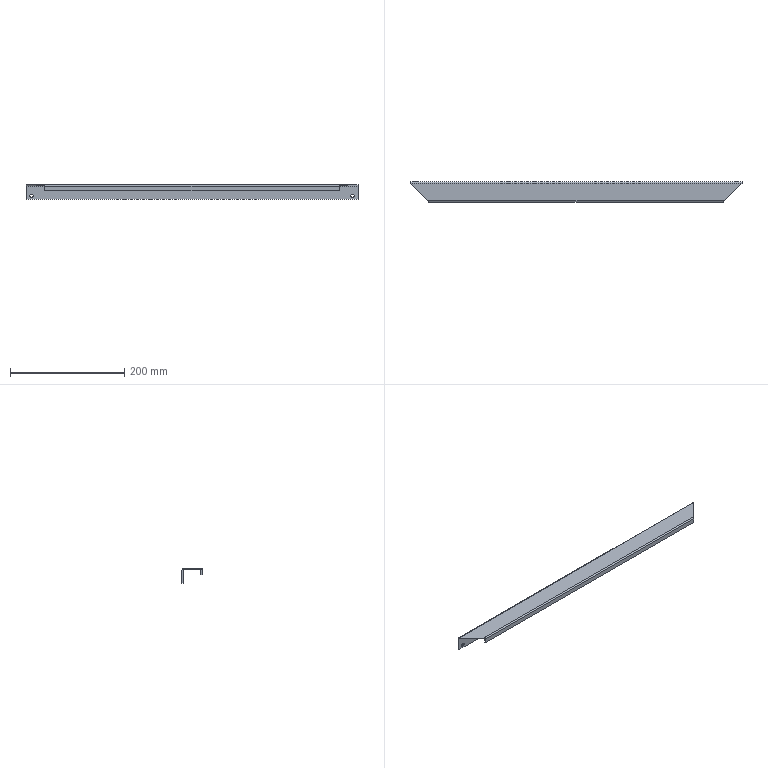Part | STEP file | Right Door Frame 3 | 1 solid | 24 faces | box 580 x 35 x 25 mm | volume 72212 mm3 | plane 16 | cylinder 8 | commonest cylinder face diameters 6 x4 0.2 x2 4.2 x2
STEP:
#1=CARTESIAN_POINT('',(-44.225,-2.,-11.695));
#2=VERTEX_POINT('',#1);
#3=CARTESIAN_POINT('',(-44.225,-2.,-5.695));
#4=VERTEX_POINT('',#3);
#5=CARTESIAN_POINT('',(-44.225,-2.,-8.695));
#6=DIRECTION('',(0.,1.,0.));
#7=DIRECTION('',(0.,0.,1.));
#8=AXIS2_PLACEMENT_3D('',#5,#6,#7);
#9=CIRCLE('',#8,3.);
#10=EDGE_CURVE('',#2,#4,#9,.T.);
#11=ORIENTED_EDGE('',*,*,#10,.F.);
#12=CARTESIAN_POINT('',(-44.225,0.,-11.695));
#13=VERTEX_POINT('',#12);
#14=CARTESIAN_POINT('',(-44.225,-10.,-11.695));
#15=DIRECTION('',(0.,1.,0.));
#16=VECTOR('',#15,1000.);
#17=LINE('',#14,#16);
#18=EDGE_CURVE('',#2,#13,#17,.T.);
#19=ORIENTED_EDGE('',*,*,#18,.T.);
#20=CARTESIAN_POINT('',(-44.225,0.,-5.695));
#21=VERTEX_POINT('',#20);
#22=CARTESIAN_POINT('',(-44.225,0.,-8.695));
#23=DIRECTION('',(0.,-1.,0.));
#24=DIRECTION('',(0.,0.,1.));
#25=AXIS2_PLACEMENT_3D('',#22,#23,#24);
#26=CIRCLE('',#25,3.);
#27=EDGE_CURVE('',#21,#13,#26,.T.);
#28=ORIENTED_EDGE('',*,*,#27,.F.);
#29=CARTESIAN_POINT('',(-44.225,-10.,-5.695));
#30=DIRECTION('',(0.,1.,0.));
#31=VECTOR('',#30,1000.);
#32=LINE('',#29,#31);
#33=EDGE_CURVE('',#4,#21,#32,.T.);
#34=ORIENTED_EDGE('',*,*,#33,.F.);
#35=EDGE_LOOP('',(#11,#19,#28,#34));
#36=FACE_OUTER_BOUND('',#35,.T.);
#37=CARTESIAN_POINT('',(-44.225,-10.,-8.695));
#38=DIRECTION('',(0.,1.,0.));
#39=DIRECTION('',(0.,0.,1.));
#40=AXIS2_PLACEMENT_3D('',#37,#38,#39);
#41=CYLINDRICAL_SURFACE('',#40,3.);
#42=ADVANCED_FACE('',(#36),#41,.F.);
#43=CARTESIAN_POINT('',(516.775,-2.,-11.695));
#44=VERTEX_POINT('',#43);
#45=CARTESIAN_POINT('',(516.775,-2.,-5.695));
#46=VERTEX_POINT('',#45);
#47=CARTESIAN_POINT('',(516.775,-2.,-8.695));
#48=DIRECTION('',(0.,1.,0.));
#49=DIRECTION('',(0.,0.,1.));
#50=AXIS2_PLACEMENT_3D('',#47,#48,#49);
#51=CIRCLE('',#50,3.);
#52=EDGE_CURVE('',#44,#46,#51,.T.);
#53=ORIENTED_EDGE('',*,*,#52,.F.);
#54=CARTESIAN_POINT('',(516.775,0.,-11.695));
#55=VERTEX_POINT('',#54);
#56=CARTESIAN_POINT('',(516.775,-10.,-11.695));
#57=DIRECTION('',(0.,1.,0.));
#58=VECTOR('',#57,1000.);
#59=LINE('',#56,#58);
#60=EDGE_CURVE('',#44,#55,#59,.T.);
#61=ORIENTED_EDGE('',*,*,#60,.T.);
#62=CARTESIAN_POINT('',(516.775,0.,-5.695));
#63=VERTEX_POINT('',#62);
#64=CARTESIAN_POINT('',(516.775,0.,-8.695));
#65=DIRECTION('',(0.,-1.,0.));
#66=DIRECTION('',(0.,0.,1.));
#67=AXIS2_PLACEMENT_3D('',#64,#65,#66);
#68=CIRCLE('',#67,3.);
#69=EDGE_CURVE('',#63,#55,#68,.T.);
#70=ORIENTED_EDGE('',*,*,#69,.F.);
#71=CARTESIAN_POINT('',(516.775,-10.,-5.695));
#72=DIRECTION('',(0.,1.,0.));
#73=VECTOR('',#72,1000.);
#74=LINE('',#71,#73);
#75=EDGE_CURVE('',#46,#63,#74,.T.);
#76=ORIENTED_EDGE('',*,*,#75,.F.);
#77=EDGE_LOOP('',(#53,#61,#70,#76));
#78=FACE_OUTER_BOUND('',#77,.T.);
#79=CARTESIAN_POINT('',(516.775,-10.,-8.695));
#80=DIRECTION('',(0.,1.,0.));
#81=DIRECTION('',(0.,0.,1.));
#82=AXIS2_PLACEMENT_3D('',#79,#80,#81);
#83=CYLINDRICAL_SURFACE('',#82,3.);
#84=ADVANCED_FACE('',(#78),#83,.F.);
#85=CARTESIAN_POINT('',(526.275,-2.1,10.305));
#86=VERTEX_POINT('',#85);
#87=CARTESIAN_POINT('',(-53.725,-2.1,10.305));
#88=VERTEX_POINT('',#87);
#89=CARTESIAN_POINT('',(0.,-2.1,10.305));
#90=DIRECTION('',(-1.,0.,0.));
#91=VECTOR('',#90,1000.);
#92=LINE('',#89,#91);
#93=EDGE_CURVE('',#86,#88,#92,.T.);
#94=ORIENTED_EDGE('',*,*,#93,.T.);
#95=CARTESIAN_POINT('',(-53.725,-2.2,10.305));
#96=VERTEX_POINT('',#95);
#97=CARTESIAN_POINT('',(-53.725,-2.,10.305));
#98=DIRECTION('',(0.,1.,0.));
#99=VECTOR('',#98,1000.);
#100=LINE('',#97,#99);
#101=EDGE_CURVE('',#96,#88,#100,.T.);
#102=ORIENTED_EDGE('',*,*,#101,.F.);
#103=CARTESIAN_POINT('',(-20.925,-35.,10.305));
#104=VERTEX_POINT('',#103);
#105=CARTESIAN_POINT('',(-53.725,-2.2,10.305));
#106=DIRECTION('',(0.7071,-0.7071,0.));
#107=VECTOR('',#106,1000.);
#108=LINE('',#105,#107);
#109=EDGE_CURVE('',#96,#104,#108,.T.);
#110=ORIENTED_EDGE('',*,*,#109,.T.);
#111=CARTESIAN_POINT('',(-20.925,-32.9,10.305));
#112=VERTEX_POINT('',#111);
#113=CARTESIAN_POINT('',(-20.925,0.,10.305));
#114=DIRECTION('',(0.,1.,0.));
#115=VECTOR('',#114,1000.);
#116=LINE('',#113,#115);
#117=EDGE_CURVE('',#104,#112,#116,.T.);
#118=ORIENTED_EDGE('',*,*,#117,.T.);
#119=CARTESIAN_POINT('',(493.475,-32.9,10.305));
#120=VERTEX_POINT('',#119);
#121=CARTESIAN_POINT('',(0.,-32.9,10.305));
#122=DIRECTION('',(1.,0.,0.));
#123=VECTOR('',#122,1000.);
#124=LINE('',#121,#123);
#125=EDGE_CURVE('',#112,#120,#124,.T.);
#126=ORIENTED_EDGE('',*,*,#125,.T.);
#127=CARTESIAN_POINT('',(493.475,-35.,10.305));
#128=VERTEX_POINT('',#127);
#129=CARTESIAN_POINT('',(493.475,0.,10.305));
#130=DIRECTION('',(0.,-1.,0.));
#131=VECTOR('',#130,1000.);
#132=LINE('',#129,#131);
#133=EDGE_CURVE('',#120,#128,#132,.T.);
#134=ORIENTED_EDGE('',*,*,#133,.T.);
#135=CARTESIAN_POINT('',(526.275,-2.2,10.305));
#136=VERTEX_POINT('',#135);
#137=CARTESIAN_POINT('',(493.475,-35.,10.305));
#138=DIRECTION('',(0.7071,0.7071,0.));
#139=VECTOR('',#138,1000.);
#140=LINE('',#137,#139);
#141=EDGE_CURVE('',#128,#136,#140,.T.);
#142=ORIENTED_EDGE('',*,*,#141,.T.);
#143=CARTESIAN_POINT('',(526.275,-35.,10.305));
#144=DIRECTION('',(0.,-1.,0.));
#145=VECTOR('',#144,1000.);
#146=LINE('',#143,#145);
#147=EDGE_CURVE('',#86,#136,#146,.T.);
#148=ORIENTED_EDGE('',*,*,#147,.F.);
#149=EDGE_LOOP('',(#94,#102,#110,#118,#126,#134,#142,#148));
#150=FACE_OUTER_BOUND('',#149,.T.);
#151=CARTESIAN_POINT('',(0.,0.,10.305));
#152=DIRECTION('',(0.,0.,1.));
#153=DIRECTION('',(0.,-1.,0.));
#154=AXIS2_PLACEMENT_3D('',#151,#152,#153);
#155=PLANE('',#154);
#156=ADVANCED_FACE('',(#150),#155,.T.);
#157=ORIENTED_EDGE('',*,*,#93,.F.);
#158=CARTESIAN_POINT('',(526.275,0.,8.205));
#159=VERTEX_POINT('',#158);
#160=CARTESIAN_POINT('',(526.275,-2.1,8.205));
#161=DIRECTION('',(-1.,0.,0.));
#162=DIRECTION('',(0.,0.,1.));
#163=AXIS2_PLACEMENT_3D('',#160,#161,#162);
#164=CIRCLE('',#163,2.1);
#165=EDGE_CURVE('',#86,#159,#164,.T.);
#166=ORIENTED_EDGE('',*,*,#165,.T.);
#167=CARTESIAN_POINT('',(-53.725,0.,8.205));
#168=VERTEX_POINT('',#167);
#169=CARTESIAN_POINT('',(-53.725,0.,8.205));
#170=DIRECTION('',(-1.,0.,0.));
#171=VECTOR('',#170,1000.);
#172=LINE('',#169,#171);
#173=EDGE_CURVE('',#159,#168,#172,.T.);
#174=ORIENTED_EDGE('',*,*,#173,.T.);
#175=CARTESIAN_POINT('',(-53.725,-2.1,8.205));
#176=DIRECTION('',(1.,0.,0.));
#177=DIRECTION('',(0.,0.,1.));
#178=AXIS2_PLACEMENT_3D('',#175,#176,#177);
#179=CIRCLE('',#178,2.1);
#180=EDGE_CURVE('',#168,#88,#179,.T.);
#181=ORIENTED_EDGE('',*,*,#180,.T.);
#182=EDGE_LOOP('',(#157,#166,#174,#181));
#183=FACE_OUTER_BOUND('',#182,.T.);
#184=CARTESIAN_POINT('',(-53.725,-2.1,8.205));
#185=DIRECTION('',(-1.,0.,0.));
#186=DIRECTION('',(0.,0.,1.));
#187=AXIS2_PLACEMENT_3D('',#184,#185,#186);
#188=CYLINDRICAL_SURFACE('',#187,2.1);
#189=ADVANCED_FACE('',(#183),#188,.T.);
#190=CARTESIAN_POINT('',(493.475,-35.,8.305));
#191=VERTEX_POINT('',#190);
#192=CARTESIAN_POINT('',(493.475,-35.,10.305));
#193=DIRECTION('',(0.,0.,1.));
#194=VECTOR('',#193,1000.);
#195=LINE('',#192,#194);
#196=EDGE_CURVE('',#191,#128,#195,.T.);
#197=ORIENTED_EDGE('',*,*,#196,.F.);
#198=CARTESIAN_POINT('',(526.275,-2.2,8.305));
#199=VERTEX_POINT('',#198);
#200=CARTESIAN_POINT('',(526.275,-2.2,8.305));
#201=DIRECTION('',(-0.7071,-0.7071,0.));
#202=VECTOR('',#201,1000.);
#203=LINE('',#200,#202);
#204=EDGE_CURVE('',#199,#191,#203,.T.);
#205=ORIENTED_EDGE('',*,*,#204,.F.);
#206=CARTESIAN_POINT('',(526.275,-2.2,10.305));
#207=DIRECTION('',(0.,0.,-1.));
#208=VECTOR('',#207,1000.);
#209=LINE('',#206,#208);
#210=EDGE_CURVE('',#136,#199,#209,.T.);
#211=ORIENTED_EDGE('',*,*,#210,.F.);
#212=ORIENTED_EDGE('',*,*,#141,.F.);
#213=EDGE_LOOP('',(#197,#205,#211,#212));
#214=FACE_OUTER_BOUND('',#213,.T.);
#215=CARTESIAN_POINT('',(526.275,-2.2,10.305));
#216=DIRECTION('',(-0.7071,0.7071,0.));
#217=DIRECTION('',(-0.7071,-0.7071,0.));
#218=AXIS2_PLACEMENT_3D('',#215,#216,#217);
#219=PLANE('',#218);
#220=ADVANCED_FACE('',(#214),#219,.F.);
#221=CARTESIAN_POINT('',(493.475,-34.998,8.305));
#222=VERTEX_POINT('',#221);
#223=CARTESIAN_POINT('',(493.475,-32.9,8.305));
#224=DIRECTION('',(0.,-1.,0.));
#225=VECTOR('',#224,1000.);
#226=LINE('',#223,#225);
#227=EDGE_CURVE('',#222,#191,#226,.T.);
#228=ORIENTED_EDGE('',*,*,#227,.T.);
#229=ORIENTED_EDGE('',*,*,#196,.T.);
#230=ORIENTED_EDGE('',*,*,#133,.F.);
#231=CARTESIAN_POINT('',(493.475,-32.9,8.205));
#232=DIRECTION('',(1.,0.,0.));
#233=DIRECTION('',(0.,0.,1.));
#234=AXIS2_PLACEMENT_3D('',#231,#232,#233);
#235=CIRCLE('',#234,2.1);
#236=EDGE_CURVE('',#120,#222,#235,.T.);
#237=ORIENTED_EDGE('',*,*,#236,.T.);
#238=EDGE_LOOP('',(#228,#229,#230,#237));
#239=FACE_OUTER_BOUND('',#238,.T.);
#240=CARTESIAN_POINT('',(493.475,-32.9,8.305));
#241=DIRECTION('',(-1.,0.,0.));
#242=DIRECTION('',(0.,-1.,0.));
#243=AXIS2_PLACEMENT_3D('',#240,#241,#242);
#244=PLANE('',#243);
#245=ADVANCED_FACE('',(#239),#244,.T.);
#246=CARTESIAN_POINT('',(493.475,-35.,8.205));
#247=VERTEX_POINT('',#246);
#248=CARTESIAN_POINT('',(493.475,-32.9,8.205));
#249=DIRECTION('',(1.,0.,0.));
#250=DIRECTION('',(0.,0.,-1.));
#251=AXIS2_PLACEMENT_3D('',#248,#249,#250);
#252=CIRCLE('',#251,2.1);
#253=EDGE_CURVE('',#222,#247,#252,.T.);
#254=ORIENTED_EDGE('',*,*,#253,.F.);
#255=ORIENTED_EDGE('',*,*,#236,.F.);
#256=ORIENTED_EDGE('',*,*,#125,.F.);
#257=CARTESIAN_POINT('',(-20.925,-34.998,8.305));
#258=VERTEX_POINT('',#257);
#259=CARTESIAN_POINT('',(-20.925,-32.9,8.205));
#260=DIRECTION('',(1.,0.,0.));
#261=DIRECTION('',(0.,0.,1.));
#262=AXIS2_PLACEMENT_3D('',#259,#260,#261);
#263=CIRCLE('',#262,2.1);
#264=EDGE_CURVE('',#112,#258,#263,.T.);
#265=ORIENTED_EDGE('',*,*,#264,.T.);
#266=CARTESIAN_POINT('',(-20.925,-35.,8.205));
#267=VERTEX_POINT('',#266);
#268=CARTESIAN_POINT('',(-20.925,-32.9,8.205));
#269=DIRECTION('',(1.,0.,0.));
#270=DIRECTION('',(0.,0.,1.));
#271=AXIS2_PLACEMENT_3D('',#268,#269,#270);
#272=CIRCLE('',#271,2.1);
#273=EDGE_CURVE('',#258,#267,#272,.T.);
#274=ORIENTED_EDGE('',*,*,#273,.T.);
#275=CARTESIAN_POINT('',(-20.925,-35.,8.205));
#276=DIRECTION('',(1.,0.,0.));
#277=VECTOR('',#276,1000.);
#278=LINE('',#275,#277);
#279=EDGE_CURVE('',#267,#247,#278,.T.);
#280=ORIENTED_EDGE('',*,*,#279,.T.);
#281=EDGE_LOOP('',(#254,#255,#256,#265,#274,#280));
#282=FACE_OUTER_BOUND('',#281,.T.);
#283=CARTESIAN_POINT('',(-20.925,-32.9,8.205));
#284=DIRECTION('',(-1.,0.,0.));
#285=DIRECTION('',(0.,0.,1.));
#286=AXIS2_PLACEMENT_3D('',#283,#284,#285);
#287=CYLINDRICAL_SURFACE('',#286,2.1);
#288=ADVANCED_FACE('',(#282),#287,.T.);
#289=ORIENTED_EDGE('',*,*,#117,.F.);
#290=CARTESIAN_POINT('',(-20.925,-35.,8.305));
#291=VERTEX_POINT('',#290);
#292=CARTESIAN_POINT('',(-20.925,-35.,8.305));
#293=DIRECTION('',(0.,0.,-1.));
#294=VECTOR('',#293,1000.);
#295=LINE('',#292,#294);
#296=EDGE_CURVE('',#104,#291,#295,.T.);
#297=ORIENTED_EDGE('',*,*,#296,.T.);
#298=CARTESIAN_POINT('',(-20.925,-35.,8.305));
#299=DIRECTION('',(0.,1.,0.));
#300=VECTOR('',#299,1000.);
#301=LINE('',#298,#300);
#302=EDGE_CURVE('',#291,#258,#301,.T.);
#303=ORIENTED_EDGE('',*,*,#302,.T.);
#304=ORIENTED_EDGE('',*,*,#264,.F.);
#305=EDGE_LOOP('',(#289,#297,#303,#304));
#306=FACE_OUTER_BOUND('',#305,.T.);
#307=CARTESIAN_POINT('',(-20.925,-35.,8.305));
#308=DIRECTION('',(1.,0.,0.));
#309=DIRECTION('',(0.,1.,0.));
#310=AXIS2_PLACEMENT_3D('',#307,#308,#309);
#311=PLANE('',#310);
#312=ADVANCED_FACE('',(#306),#311,.T.);
#313=CARTESIAN_POINT('',(-53.725,-2.2,8.305));
#314=VERTEX_POINT('',#313);
#315=CARTESIAN_POINT('',(-53.725,-2.2,10.305));
#316=DIRECTION('',(0.,0.,1.));
#317=VECTOR('',#316,1000.);
#318=LINE('',#315,#317);
#319=EDGE_CURVE('',#314,#96,#318,.T.);
#320=ORIENTED_EDGE('',*,*,#319,.F.);
#321=CARTESIAN_POINT('',(-20.925,-35.,8.305));
#322=DIRECTION('',(-0.7071,0.7071,0.));
#323=VECTOR('',#322,1000.);
#324=LINE('',#321,#323);
#325=EDGE_CURVE('',#291,#314,#324,.T.);
#326=ORIENTED_EDGE('',*,*,#325,.F.);
#327=ORIENTED_EDGE('',*,*,#296,.F.);
#328=ORIENTED_EDGE('',*,*,#109,.F.);
#329=EDGE_LOOP('',(#320,#326,#327,#328));
#330=FACE_OUTER_BOUND('',#329,.T.);
#331=CARTESIAN_POINT('',(-20.925,-35.,10.305));
#332=DIRECTION('',(0.7071,0.7071,0.));
#333=DIRECTION('',(-0.7071,0.7071,0.));
#334=AXIS2_PLACEMENT_3D('',#331,#332,#333);
#335=PLANE('',#334);
#336=ADVANCED_FACE('',(#330),#335,.F.);
#337=CARTESIAN_POINT('',(526.275,-2.1,8.305));
#338=VERTEX_POINT('',#337);
#339=CARTESIAN_POINT('',(526.275,-2.,8.205));
#340=VERTEX_POINT('',#339);
#341=CARTESIAN_POINT('',(526.275,-2.1,8.205));
#342=DIRECTION('',(-1.,0.,0.));
#343=DIRECTION('',(0.,0.,1.));
#344=AXIS2_PLACEMENT_3D('',#341,#342,#343);
#345=CIRCLE('',#344,0.1);
#346=EDGE_CURVE('',#338,#340,#345,.T.);
#347=ORIENTED_EDGE('',*,*,#346,.T.);
#348=CARTESIAN_POINT('',(526.275,-2.,-14.695));
#349=VERTEX_POINT('',#348);
#350=CARTESIAN_POINT('',(526.275,-2.,-14.695));
#351=DIRECTION('',(0.,0.,-1.));
#352=VECTOR('',#351,1000.);
#353=LINE('',#350,#352);
#354=EDGE_CURVE('',#340,#349,#353,.T.);
#355=ORIENTED_EDGE('',*,*,#354,.T.);
#356=CARTESIAN_POINT('',(526.275,0.,-14.695));
#357=VERTEX_POINT('',#356);
#358=CARTESIAN_POINT('',(526.275,-2.,-14.695));
#359=DIRECTION('',(0.,1.,0.));
#360=VECTOR('',#359,1000.);
#361=LINE('',#358,#360);
#362=EDGE_CURVE('',#349,#357,#361,.T.);
#363=ORIENTED_EDGE('',*,*,#362,.T.);
#364=CARTESIAN_POINT('',(526.275,0.,0.));
#365=DIRECTION('',(0.,0.,-1.));
#366=VECTOR('',#365,1000.);
#367=LINE('',#364,#366);
#368=EDGE_CURVE('',#159,#357,#367,.T.);
#369=ORIENTED_EDGE('',*,*,#368,.F.);
#370=ORIENTED_EDGE('',*,*,#165,.F.);
#371=ORIENTED_EDGE('',*,*,#147,.T.);
#372=ORIENTED_EDGE('',*,*,#210,.T.);
#373=CARTESIAN_POINT('',(526.275,0.,8.305));
#374=DIRECTION('',(0.,1.,0.));
#375=VECTOR('',#374,1000.);
#376=LINE('',#373,#375);
#377=EDGE_CURVE('',#199,#338,#376,.T.);
#378=ORIENTED_EDGE('',*,*,#377,.T.);
#379=EDGE_LOOP('',(#347,#355,#363,#369,#370,#371,#372,#378));
#380=FACE_OUTER_BOUND('',#379,.T.);
#381=CARTESIAN_POINT('',(526.275,-2.1,8.205));
#382=DIRECTION('',(1.,0.,0.));
#383=DIRECTION('',(0.,0.,-1.));
#384=AXIS2_PLACEMENT_3D('',#381,#382,#383);
#385=PLANE('',#384);
#386=ADVANCED_FACE('',(#380),#385,.T.);
#387=CARTESIAN_POINT('',(-53.725,-2.,8.205));
#388=VERTEX_POINT('',#387);
#389=CARTESIAN_POINT('',(-53.725,-2.1,8.305));
#390=VERTEX_POINT('',#389);
#391=CARTESIAN_POINT('',(-53.725,-2.1,8.205));
#392=DIRECTION('',(1.,0.,0.));
#393=DIRECTION('',(0.,0.,1.));
#394=AXIS2_PLACEMENT_3D('',#391,#392,#393);
#395=CIRCLE('',#394,0.1);
#396=EDGE_CURVE('',#388,#390,#395,.T.);
#397=ORIENTED_EDGE('',*,*,#396,.T.);
#398=CARTESIAN_POINT('',(-53.725,0.,8.305));
#399=DIRECTION('',(0.,-1.,0.));
#400=VECTOR('',#399,1000.);
#401=LINE('',#398,#400);
#402=EDGE_CURVE('',#390,#314,#401,.T.);
#403=ORIENTED_EDGE('',*,*,#402,.T.);
#404=ORIENTED_EDGE('',*,*,#319,.T.);
#405=ORIENTED_EDGE('',*,*,#101,.T.);
#406=ORIENTED_EDGE('',*,*,#180,.F.);
#407=CARTESIAN_POINT('',(-53.725,0.,-14.695));
#408=VERTEX_POINT('',#407);
#409=CARTESIAN_POINT('',(-53.725,0.,0.));
#410=DIRECTION('',(0.,0.,1.));
#411=VECTOR('',#410,1000.);
#412=LINE('',#409,#411);
#413=EDGE_CURVE('',#408,#168,#412,.T.);
#414=ORIENTED_EDGE('',*,*,#413,.F.);
#415=CARTESIAN_POINT('',(-53.725,-2.,-14.695));
#416=VERTEX_POINT('',#415);
#417=CARTESIAN_POINT('',(-53.725,-2.,-14.695));
#418=DIRECTION('',(0.,-1.,0.));
#419=VECTOR('',#418,1000.);
#420=LINE('',#417,#419);
#421=EDGE_CURVE('',#408,#416,#420,.T.);
#422=ORIENTED_EDGE('',*,*,#421,.T.);
#423=CARTESIAN_POINT('',(-53.725,-2.,-14.695));
#424=DIRECTION('',(0.,0.,1.));
#425=VECTOR('',#424,1000.);
#426=LINE('',#423,#425);
#427=EDGE_CURVE('',#416,#388,#426,.T.);
#428=ORIENTED_EDGE('',*,*,#427,.T.);
#429=EDGE_LOOP('',(#397,#403,#404,#405,#406,#414,#422,#428));
#430=FACE_OUTER_BOUND('',#429,.T.);
#431=CARTESIAN_POINT('',(-53.725,-2.1,8.205));
#432=DIRECTION('',(1.,0.,0.));
#433=DIRECTION('',(0.,0.,-1.));
#434=AXIS2_PLACEMENT_3D('',#431,#432,#433);
#435=PLANE('',#434);
#436=ADVANCED_FACE('',(#430),#435,.F.);
#437=ORIENTED_EDGE('',*,*,#368,.T.);
#438=CARTESIAN_POINT('',(0.,0.,-14.695));
#439=DIRECTION('',(-1.,0.,0.));
#440=VECTOR('',#439,1000.);
#441=LINE('',#438,#440);
#442=EDGE_CURVE('',#357,#408,#441,.T.);
#443=ORIENTED_EDGE('',*,*,#442,.T.);
#444=ORIENTED_EDGE('',*,*,#413,.T.);
#445=ORIENTED_EDGE('',*,*,#173,.F.);
#446=EDGE_LOOP('',(#437,#443,#444,#445));
#447=FACE_OUTER_BOUND('',#446,.T.);
#448=ORIENTED_EDGE('',*,*,#27,.T.);
#449=CARTESIAN_POINT('',(-44.225,0.,-8.695));
#450=DIRECTION('',(0.,-1.,0.));
#451=DIRECTION('',(0.,0.,1.));
#452=AXIS2_PLACEMENT_3D('',#449,#450,#451);
#453=CIRCLE('',#452,3.);
#454=EDGE_CURVE('',#13,#21,#453,.T.);
#455=ORIENTED_EDGE('',*,*,#454,.T.);
#456=EDGE_LOOP('',(#448,#455));
#457=FACE_BOUND('',#456,.T.);
#458=ORIENTED_EDGE('',*,*,#69,.T.);
#459=CARTESIAN_POINT('',(516.775,0.,-8.695));
#460=DIRECTION('',(0.,-1.,0.));
#461=DIRECTION('',(0.,0.,1.));
#462=AXIS2_PLACEMENT_3D('',#459,#460,#461);
#463=CIRCLE('',#462,3.);
#464=EDGE_CURVE('',#55,#63,#463,.T.);
#465=ORIENTED_EDGE('',*,*,#464,.T.);
#466=EDGE_LOOP('',(#458,#465));
#467=FACE_BOUND('',#466,.T.);
#468=CARTESIAN_POINT('',(0.,0.,0.));
#469=DIRECTION('',(0.,1.,0.));
#470=DIRECTION('',(0.,0.,1.));
#471=AXIS2_PLACEMENT_3D('',#468,#469,#470);
#472=PLANE('',#471);
#473=ADVANCED_FACE('',(#447,#457,#467),#472,.T.);
#474=ORIENTED_EDGE('',*,*,#325,.T.);
#475=ORIENTED_EDGE('',*,*,#402,.F.);
#476=CARTESIAN_POINT('',(0.,-2.1,8.305));
#477=DIRECTION('',(-1.,0.,0.));
#478=VECTOR('',#477,1000.);
#479=LINE('',#476,#478);
#480=EDGE_CURVE('',#338,#390,#479,.T.);
#481=ORIENTED_EDGE('',*,*,#480,.F.);
#482=ORIENTED_EDGE('',*,*,#377,.F.);
#483=ORIENTED_EDGE('',*,*,#204,.T.);
#484=ORIENTED_EDGE('',*,*,#227,.F.);
#485=CARTESIAN_POINT('',(493.475,-32.9,8.305));
#486=VERTEX_POINT('',#485);
#487=CARTESIAN_POINT('',(493.475,0.,8.305));
#488=DIRECTION('',(0.,-1.,0.));
#489=VECTOR('',#488,1000.);
#490=LINE('',#487,#489);
#491=EDGE_CURVE('',#486,#222,#490,.T.);
#492=ORIENTED_EDGE('',*,*,#491,.F.);
#493=CARTESIAN_POINT('',(-20.925,-32.9,8.305));
#494=VERTEX_POINT('',#493);
#495=CARTESIAN_POINT('',(0.,-32.9,8.305));
#496=DIRECTION('',(1.,0.,0.));
#497=VECTOR('',#496,1000.);
#498=LINE('',#495,#497);
#499=EDGE_CURVE('',#494,#486,#498,.T.);
#500=ORIENTED_EDGE('',*,*,#499,.F.);
#501=CARTESIAN_POINT('',(-20.925,0.,8.305));
#502=DIRECTION('',(0.,1.,0.));
#503=VECTOR('',#502,1000.);
#504=LINE('',#501,#503);
#505=EDGE_CURVE('',#258,#494,#504,.T.);
#506=ORIENTED_EDGE('',*,*,#505,.F.);
#507=ORIENTED_EDGE('',*,*,#302,.F.);
#508=EDGE_LOOP('',(#474,#475,#481,#482,#483,#484,#492,#500,#506,#507));
#509=FACE_OUTER_BOUND('',#508,.T.);
#510=CARTESIAN_POINT('',(0.,0.,8.305));
#511=DIRECTION('',(0.,0.,1.));
#512=DIRECTION('',(0.,-1.,0.));
#513=AXIS2_PLACEMENT_3D('',#510,#511,#512);
#514=PLANE('',#513);
#515=ADVANCED_FACE('',(#509),#514,.F.);
#516=CARTESIAN_POINT('',(-20.925,-35.,0.3046));
#517=VERTEX_POINT('',#516);
#518=CARTESIAN_POINT('',(-20.925,-35.,0.));
#519=DIRECTION('',(0.,0.,-1.));
#520=VECTOR('',#519,1000.);
#521=LINE('',#518,#520);
#522=EDGE_CURVE('',#267,#517,#521,.T.);
#523=ORIENTED_EDGE('',*,*,#522,.T.);
#524=CARTESIAN_POINT('',(493.475,-35.,0.3046));
#525=VERTEX_POINT('',#524);
#526=CARTESIAN_POINT('',(0.,-35.,0.3046));
#527=DIRECTION('',(1.,0.,0.));
#528=VECTOR('',#527,1000.);
#529=LINE('',#526,#528);
#530=EDGE_CURVE('',#517,#525,#529,.T.);
#531=ORIENTED_EDGE('',*,*,#530,.T.);
#532=CARTESIAN_POINT('',(493.475,-35.,0.));
#533=DIRECTION('',(0.,0.,1.));
#534=VECTOR('',#533,1000.);
#535=LINE('',#532,#534);
#536=EDGE_CURVE('',#525,#247,#535,.T.);
#537=ORIENTED_EDGE('',*,*,#536,.T.);
#538=ORIENTED_EDGE('',*,*,#279,.F.);
#539=EDGE_LOOP('',(#523,#531,#537,#538));
#540=FACE_OUTER_BOUND('',#539,.T.);
#541=CARTESIAN_POINT('',(0.,-35.,0.));
#542=DIRECTION('',(0.,-1.,0.));
#543=DIRECTION('',(0.,0.,-1.));
#544=AXIS2_PLACEMENT_3D('',#541,#542,#543);
#545=PLANE('',#544);
#546=ADVANCED_FACE('',(#540),#545,.T.);
#547=CARTESIAN_POINT('',(-53.725,-2.,-14.695));
#548=DIRECTION('',(-1.,0.,0.));
#549=VECTOR('',#548,1000.);
#550=LINE('',#547,#549);
#551=EDGE_CURVE('',#349,#416,#550,.T.);
#552=ORIENTED_EDGE('',*,*,#551,.T.);
#553=ORIENTED_EDGE('',*,*,#421,.F.);
#554=ORIENTED_EDGE('',*,*,#442,.F.);
#555=ORIENTED_EDGE('',*,*,#362,.F.);
#556=EDGE_LOOP('',(#552,#553,#554,#555));
#557=FACE_OUTER_BOUND('',#556,.T.);
#558=CARTESIAN_POINT('',(-53.725,-2.,-14.695));
#559=DIRECTION('',(0.,0.,-1.));
#560=DIRECTION('',(-1.,0.,0.));
#561=AXIS2_PLACEMENT_3D('',#558,#559,#560);
#562=PLANE('',#561);
#563=ADVANCED_FACE('',(#557),#562,.T.);
#564=ORIENTED_EDGE('',*,*,#18,.F.);
#565=CARTESIAN_POINT('',(-44.225,-2.,-8.695));
#566=DIRECTION('',(0.,1.,0.));
#567=DIRECTION('',(0.,0.,1.));
#568=AXIS2_PLACEMENT_3D('',#565,#566,#567);
#569=CIRCLE('',#568,3.);
#570=EDGE_CURVE('',#4,#2,#569,.T.);
#571=ORIENTED_EDGE('',*,*,#570,.F.);
#572=ORIENTED_EDGE('',*,*,#33,.T.);
#573=ORIENTED_EDGE('',*,*,#454,.F.);
#574=EDGE_LOOP('',(#564,#571,#572,#573));
#575=FACE_OUTER_BOUND('',#574,.T.);
#576=CARTESIAN_POINT('',(-44.225,-10.,-8.695));
#577=DIRECTION('',(0.,1.,0.));
#578=DIRECTION('',(0.,0.,1.));
#579=AXIS2_PLACEMENT_3D('',#576,#577,#578);
#580=CYLINDRICAL_SURFACE('',#579,3.);
#581=ADVANCED_FACE('',(#575),#580,.F.);
#582=ORIENTED_EDGE('',*,*,#60,.F.);
#583=CARTESIAN_POINT('',(516.775,-2.,-8.695));
#584=DIRECTION('',(0.,1.,0.));
#585=DIRECTION('',(0.,0.,1.));
#586=AXIS2_PLACEMENT_3D('',#583,#584,#585);
#587=CIRCLE('',#586,3.);
#588=EDGE_CURVE('',#46,#44,#587,.T.);
#589=ORIENTED_EDGE('',*,*,#588,.F.);
#590=ORIENTED_EDGE('',*,*,#75,.T.);
#591=ORIENTED_EDGE('',*,*,#464,.F.);
#592=EDGE_LOOP('',(#582,#589,#590,#591));
#593=FACE_OUTER_BOUND('',#592,.T.);
#594=CARTESIAN_POINT('',(516.775,-10.,-8.695));
#595=DIRECTION('',(0.,1.,0.));
#596=DIRECTION('',(0.,0.,1.));
#597=AXIS2_PLACEMENT_3D('',#594,#595,#596);
#598=CYLINDRICAL_SURFACE('',#597,3.);
#599=ADVANCED_FACE('',(#593),#598,.F.);
#600=ORIENTED_EDGE('',*,*,#346,.F.);
#601=ORIENTED_EDGE('',*,*,#480,.T.);
#602=ORIENTED_EDGE('',*,*,#396,.F.);
#603=CARTESIAN_POINT('',(-53.725,-2.,8.205));
#604=DIRECTION('',(-1.,0.,0.));
#605=VECTOR('',#604,1000.);
#606=LINE('',#603,#605);
#607=EDGE_CURVE('',#340,#388,#606,.T.);
#608=ORIENTED_EDGE('',*,*,#607,.F.);
#609=EDGE_LOOP('',(#600,#601,#602,#608));
#610=FACE_OUTER_BOUND('',#609,.T.);
#611=CARTESIAN_POINT('',(-53.725,-2.1,8.205));
#612=DIRECTION('',(-1.,0.,0.));
#613=DIRECTION('',(0.,0.,1.));
#614=AXIS2_PLACEMENT_3D('',#611,#612,#613);
#615=CYLINDRICAL_SURFACE('',#614,0.1);
#616=ADVANCED_FACE('',(#610),#615,.F.);
#617=ORIENTED_EDGE('',*,*,#253,.T.);
#618=ORIENTED_EDGE('',*,*,#536,.F.);
#619=CARTESIAN_POINT('',(493.475,-33.,0.3046));
#620=VERTEX_POINT('',#619);
#621=CARTESIAN_POINT('',(493.475,-35.,0.3046));
#622=DIRECTION('',(0.,-1.,0.));
#623=VECTOR('',#622,1000.);
#624=LINE('',#621,#623);
#625=EDGE_CURVE('',#620,#525,#624,.T.);
#626=ORIENTED_EDGE('',*,*,#625,.F.);
#627=CARTESIAN_POINT('',(493.475,-33.,8.205));
#628=VERTEX_POINT('',#627);
#629=CARTESIAN_POINT('',(493.475,-33.,0.3046));
#630=DIRECTION('',(0.,0.,1.));
#631=VECTOR('',#630,1000.);
#632=LINE('',#629,#631);
#633=EDGE_CURVE('',#620,#628,#632,.T.);
#634=ORIENTED_EDGE('',*,*,#633,.T.);
#635=CARTESIAN_POINT('',(493.475,-32.9,8.205));
#636=DIRECTION('',(-1.,0.,0.));
#637=DIRECTION('',(0.,0.,1.));
#638=AXIS2_PLACEMENT_3D('',#635,#636,#637);
#639=CIRCLE('',#638,0.1);
#640=EDGE_CURVE('',#628,#486,#639,.T.);
#641=ORIENTED_EDGE('',*,*,#640,.T.);
#642=ORIENTED_EDGE('',*,*,#491,.T.);
#643=EDGE_LOOP('',(#617,#618,#626,#634,#641,#642));
#644=FACE_OUTER_BOUND('',#643,.T.);
#645=CARTESIAN_POINT('',(493.475,-32.9,8.205));
#646=DIRECTION('',(1.,0.,0.));
#647=DIRECTION('',(0.,0.,-1.));
#648=AXIS2_PLACEMENT_3D('',#645,#646,#647);
#649=PLANE('',#648);
#650=ADVANCED_FACE('',(#644),#649,.T.);
#651=ORIENTED_EDGE('',*,*,#640,.F.);
#652=CARTESIAN_POINT('',(-20.925,-33.,8.205));
#653=VERTEX_POINT('',#652);
#654=CARTESIAN_POINT('',(-20.925,-33.,8.205));
#655=DIRECTION('',(1.,0.,0.));
#656=VECTOR('',#655,1000.);
#657=LINE('',#654,#656);
#658=EDGE_CURVE('',#653,#628,#657,.T.);
#659=ORIENTED_EDGE('',*,*,#658,.F.);
#660=CARTESIAN_POINT('',(-20.925,-32.9,8.205));
#661=DIRECTION('',(1.,0.,0.));
#662=DIRECTION('',(0.,0.,1.));
#663=AXIS2_PLACEMENT_3D('',#660,#661,#662);
#664=CIRCLE('',#663,0.1);
#665=EDGE_CURVE('',#494,#653,#664,.T.);
#666=ORIENTED_EDGE('',*,*,#665,.F.);
#667=ORIENTED_EDGE('',*,*,#499,.T.);
#668=EDGE_LOOP('',(#651,#659,#666,#667));
#669=FACE_OUTER_BOUND('',#668,.T.);
#670=CARTESIAN_POINT('',(-20.925,-32.9,8.205));
#671=DIRECTION('',(-1.,0.,0.));
#672=DIRECTION('',(0.,0.,1.));
#673=AXIS2_PLACEMENT_3D('',#670,#671,#672);
#674=CYLINDRICAL_SURFACE('',#673,0.1);
#675=ADVANCED_FACE('',(#669),#674,.F.);
#676=ORIENTED_EDGE('',*,*,#505,.T.);
#677=ORIENTED_EDGE('',*,*,#665,.T.);
#678=CARTESIAN_POINT('',(-20.925,-33.,0.3046));
#679=VERTEX_POINT('',#678);
#680=CARTESIAN_POINT('',(-20.925,-33.,8.305));
#681=DIRECTION('',(0.,0.,-1.));
#682=VECTOR('',#681,1000.);
#683=LINE('',#680,#682);
#684=EDGE_CURVE('',#653,#679,#683,.T.);
#685=ORIENTED_EDGE('',*,*,#684,.T.);
#686=CARTESIAN_POINT('',(-20.925,-35.,0.3046));
#687=DIRECTION('',(0.,1.,0.));
#688=VECTOR('',#687,1000.);
#689=LINE('',#686,#688);
#690=EDGE_CURVE('',#517,#679,#689,.T.);
#691=ORIENTED_EDGE('',*,*,#690,.F.);
#692=ORIENTED_EDGE('',*,*,#522,.F.);
#693=ORIENTED_EDGE('',*,*,#273,.F.);
#694=EDGE_LOOP('',(#676,#677,#685,#691,#692,#693));
#695=FACE_OUTER_BOUND('',#694,.T.);
#696=CARTESIAN_POINT('',(-20.925,-32.9,8.205));
#697=DIRECTION('',(1.,0.,0.));
#698=DIRECTION('',(0.,0.,-1.));
#699=AXIS2_PLACEMENT_3D('',#696,#697,#698);
#700=PLANE('',#699);
#701=ADVANCED_FACE('',(#695),#700,.F.);
#702=ORIENTED_EDGE('',*,*,#530,.F.);
#703=ORIENTED_EDGE('',*,*,#690,.T.);
#704=CARTESIAN_POINT('',(-20.925,-33.,0.3046));
#705=DIRECTION('',(1.,0.,0.));
#706=VECTOR('',#705,1000.);
#707=LINE('',#704,#706);
#708=EDGE_CURVE('',#679,#620,#707,.T.);
#709=ORIENTED_EDGE('',*,*,#708,.T.);
#710=ORIENTED_EDGE('',*,*,#625,.T.);
#711=EDGE_LOOP('',(#702,#703,#709,#710));
#712=FACE_OUTER_BOUND('',#711,.T.);
#713=CARTESIAN_POINT('',(-20.925,-35.,0.3046));
#714=DIRECTION('',(0.,0.,-1.));
#715=DIRECTION('',(0.,1.,0.));
#716=AXIS2_PLACEMENT_3D('',#713,#714,#715);
#717=PLANE('',#716);
#718=ADVANCED_FACE('',(#712),#717,.T.);
#719=ORIENTED_EDGE('',*,*,#427,.F.);
#720=ORIENTED_EDGE('',*,*,#551,.F.);
#721=ORIENTED_EDGE('',*,*,#354,.F.);
#722=ORIENTED_EDGE('',*,*,#607,.T.);
#723=EDGE_LOOP('',(#719,#720,#721,#722));
#724=FACE_OUTER_BOUND('',#723,.T.);
#725=ORIENTED_EDGE('',*,*,#570,.T.);
#726=ORIENTED_EDGE('',*,*,#10,.T.);
#727=EDGE_LOOP('',(#725,#726));
#728=FACE_BOUND('',#727,.T.);
#729=ORIENTED_EDGE('',*,*,#588,.T.);
#730=ORIENTED_EDGE('',*,*,#52,.T.);
#731=EDGE_LOOP('',(#729,#730));
#732=FACE_BOUND('',#731,.T.);
#733=CARTESIAN_POINT('',(0.,-2.,0.));
#734=DIRECTION('',(0.,1.,0.));
#735=DIRECTION('',(0.,0.,1.));
#736=AXIS2_PLACEMENT_3D('',#733,#734,#735);
#737=PLANE('',#736);
#738=ADVANCED_FACE('',(#724,#728,#732),#737,.F.);
#739=ORIENTED_EDGE('',*,*,#633,.F.);
#740=ORIENTED_EDGE('',*,*,#708,.F.);
#741=ORIENTED_EDGE('',*,*,#684,.F.);
#742=ORIENTED_EDGE('',*,*,#658,.T.);
#743=EDGE_LOOP('',(#739,#740,#741,#742));
#744=FACE_OUTER_BOUND('',#743,.T.);
#745=CARTESIAN_POINT('',(0.,-33.,0.));
#746=DIRECTION('',(0.,-1.,0.));
#747=DIRECTION('',(0.,0.,-1.));
#748=AXIS2_PLACEMENT_3D('',#745,#746,#747);
#749=PLANE('',#748);
#750=ADVANCED_FACE('',(#744),#749,.F.);
#751=CLOSED_SHELL('',(#42,#84,#156,#189,#220,#245,#288,#312,#336,#386,#436,#473,#515,#546,#563,#581,#599,#616,#650,#675,#701,#718,#738,#750));
#752=MANIFOLD_SOLID_BREP('',#751);
#753=CARTESIAN_POINT('',(0.,0.,0.));
#754=DIRECTION('',(0.,0.,1.));
#755=DIRECTION('',(1.,0.,0.));
#756=AXIS2_PLACEMENT_3D('',#753,#754,#755);
#757=(LENGTH_UNIT()NAMED_UNIT(*)SI_UNIT(.MILLI.,.METRE.));
#758=UNCERTAINTY_MEASURE_WITH_UNIT(LENGTH_MEASURE(0.00001),#757,'','');
#759=(NAMED_UNIT(*)PLANE_ANGLE_UNIT()SI_UNIT($,.RADIAN.));
#760=(NAMED_UNIT(*)SI_UNIT($,.STERADIAN.)SOLID_ANGLE_UNIT());
#761=(GEOMETRIC_REPRESENTATION_CONTEXT(3)GLOBAL_UNCERTAINTY_ASSIGNED_CONTEXT((#758))GLOBAL_UNIT_ASSIGNED_CONTEXT((#757,#759,#760))REPRESENTATION_CONTEXT('',''));
#762=ADVANCED_BREP_SHAPE_REPRESENTATION('',(#752,#756),#761);